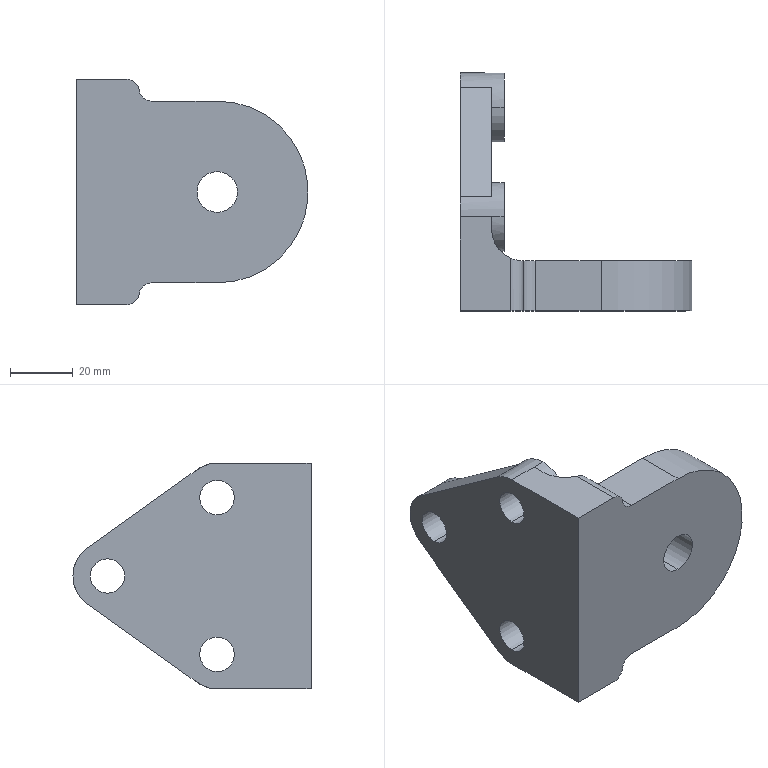Part | SolidWorks | features BaseBody 1 | 1 solid | 38 faces | box 74 x 76 x 72 mm | volume 94781 mm3 | cylinder 22 | plane 16 | commonest cylinder face diameters 11 x6 22 x6 8 x4 13 x2 36 x2 20 x1
STEP:
#1=CARTESIAN_POINT('',(45.,0.,42.5));
#2=VERTEX_POINT('',#1);
#3=CARTESIAN_POINT('',(45.,0.,29.5));
#4=VERTEX_POINT('',#3);
#5=CARTESIAN_POINT('',(45.,0.,36.));
#6=DIRECTION('',(0.,-1.,0.));
#7=DIRECTION('',(0.,0.,1.));
#8=AXIS2_PLACEMENT_3D('',#5,#6,#7);
#9=CIRCLE('',#8,6.5);
#10=EDGE_CURVE('',#2,#4,#9,.T.);
#11=ORIENTED_EDGE('',*,*,#10,.T.);
#12=CARTESIAN_POINT('',(45.,13.,29.5));
#13=VERTEX_POINT('',#12);
#14=CARTESIAN_POINT('',(45.,0.,29.5));
#15=DIRECTION('',(0.,1.,0.));
#16=VECTOR('',#15,1000.);
#17=LINE('',#14,#16);
#18=EDGE_CURVE('',#4,#13,#17,.T.);
#19=ORIENTED_EDGE('',*,*,#18,.T.);
#20=CARTESIAN_POINT('',(45.,13.,42.5));
#21=VERTEX_POINT('',#20);
#22=CARTESIAN_POINT('',(45.,13.,36.));
#23=DIRECTION('',(0.,-1.,0.));
#24=DIRECTION('',(0.,0.,1.));
#25=AXIS2_PLACEMENT_3D('',#22,#23,#24);
#26=CIRCLE('',#25,6.5);
#27=EDGE_CURVE('',#21,#13,#26,.T.);
#28=ORIENTED_EDGE('',*,*,#27,.F.);
#29=CARTESIAN_POINT('',(45.,0.,42.5));
#30=DIRECTION('',(0.,1.,0.));
#31=VECTOR('',#30,1000.);
#32=LINE('',#29,#31);
#33=EDGE_CURVE('',#2,#21,#32,.T.);
#34=ORIENTED_EDGE('',*,*,#33,.F.);
#35=EDGE_LOOP('',(#11,#19,#28,#34));
#36=FACE_OUTER_BOUND('',#35,.T.);
#37=CARTESIAN_POINT('',(45.,0.,36.));
#38=DIRECTION('',(0.,1.,0.));
#39=DIRECTION('',(0.,0.,1.));
#40=AXIS2_PLACEMENT_3D('',#37,#38,#39);
#41=CYLINDRICAL_SURFACE('',#40,6.5);
#42=ADVANCED_FACE('',(#36),#41,.F.);
#43=CARTESIAN_POINT('',(10.,30.,72.));
#44=VERTEX_POINT('',#43);
#45=CARTESIAN_POINT('',(0.,30.,72.));
#46=VERTEX_POINT('',#45);
#47=CARTESIAN_POINT('',(8.031,30.,72.));
#48=DIRECTION('',(-1.,0.,0.));
#49=VECTOR('',#48,1000.);
#50=LINE('',#47,#49);
#51=EDGE_CURVE('',#44,#46,#50,.T.);
#52=ORIENTED_EDGE('',*,*,#51,.F.);
#53=CARTESIAN_POINT('',(14.,30.,72.));
#54=VERTEX_POINT('',#53);
#55=CARTESIAN_POINT('',(0.,30.,72.));
#56=DIRECTION('',(1.,0.,0.));
#57=VECTOR('',#56,1000.);
#58=LINE('',#55,#57);
#59=EDGE_CURVE('',#44,#54,#58,.T.);
#60=ORIENTED_EDGE('',*,*,#59,.T.);
#61=CARTESIAN_POINT('',(14.,30.,50.));
#62=VERTEX_POINT('',#61);
#63=CARTESIAN_POINT('',(14.,30.,61.));
#64=DIRECTION('',(-1.,0.,0.));
#65=DIRECTION('',(0.,0.,-1.));
#66=AXIS2_PLACEMENT_3D('',#63,#64,#65);
#67=CIRCLE('',#66,11.);
#68=EDGE_CURVE('',#54,#62,#67,.T.);
#69=ORIENTED_EDGE('',*,*,#68,.T.);
#70=CARTESIAN_POINT('',(10.,30.,50.));
#71=VERTEX_POINT('',#70);
#72=CARTESIAN_POINT('',(0.,30.,50.));
#73=DIRECTION('',(1.,0.,0.));
#74=VECTOR('',#73,1000.);
#75=LINE('',#72,#74);
#76=EDGE_CURVE('',#71,#62,#75,.T.);
#77=ORIENTED_EDGE('',*,*,#76,.F.);
#78=CARTESIAN_POINT('',(10.,36.394,69.951));
#79=VERTEX_POINT('',#78);
#80=CARTESIAN_POINT('',(10.,30.,61.));
#81=DIRECTION('',(1.,0.,0.));
#82=DIRECTION('',(0.,0.,-1.));
#83=AXIS2_PLACEMENT_3D('',#80,#81,#82);
#84=CIRCLE('',#83,11.);
#85=EDGE_CURVE('',#71,#79,#84,.T.);
#86=ORIENTED_EDGE('',*,*,#85,.T.);
#87=CARTESIAN_POINT('',(0.,36.394,69.951));
#88=VERTEX_POINT('',#87);
#89=CARTESIAN_POINT('',(0.,36.394,69.951));
#90=DIRECTION('',(-1.,0.,0.));
#91=VECTOR('',#90,1000.);
#92=LINE('',#89,#91);
#93=EDGE_CURVE('',#79,#88,#92,.T.);
#94=ORIENTED_EDGE('',*,*,#93,.T.);
#95=CARTESIAN_POINT('',(0.,30.,61.));
#96=DIRECTION('',(1.,0.,0.));
#97=DIRECTION('',(0.,0.,-1.));
#98=AXIS2_PLACEMENT_3D('',#95,#96,#97);
#99=CIRCLE('',#98,11.);
#100=EDGE_CURVE('',#88,#46,#99,.T.);
#101=ORIENTED_EDGE('',*,*,#100,.T.);
#102=EDGE_LOOP('',(#52,#60,#69,#77,#86,#94,#101));
#103=FACE_OUTER_BOUND('',#102,.T.);
#104=CARTESIAN_POINT('',(0.,30.,61.));
#105=DIRECTION('',(1.,0.,0.));
#106=DIRECTION('',(0.,0.,-1.));
#107=AXIS2_PLACEMENT_3D('',#104,#105,#106);
#108=CYLINDRICAL_SURFACE('',#107,11.);
#109=ADVANCED_FACE('',(#103),#108,.T.);
#110=CARTESIAN_POINT('',(0.,65.,30.5));
#111=VERTEX_POINT('',#110);
#112=CARTESIAN_POINT('',(0.,65.,41.5));
#113=VERTEX_POINT('',#112);
#114=CARTESIAN_POINT('',(0.,65.,36.));
#115=DIRECTION('',(-1.,0.,0.));
#116=DIRECTION('',(0.,0.,-1.));
#117=AXIS2_PLACEMENT_3D('',#114,#115,#116);
#118=CIRCLE('',#117,5.5);
#119=EDGE_CURVE('',#111,#113,#118,.T.);
#120=ORIENTED_EDGE('',*,*,#119,.T.);
#121=CARTESIAN_POINT('',(14.,65.,41.5));
#122=VERTEX_POINT('',#121);
#123=CARTESIAN_POINT('',(0.,65.,41.5));
#124=DIRECTION('',(1.,0.,0.));
#125=VECTOR('',#124,1000.);
#126=LINE('',#123,#125);
#127=EDGE_CURVE('',#113,#122,#126,.T.);
#128=ORIENTED_EDGE('',*,*,#127,.T.);
#129=CARTESIAN_POINT('',(14.,65.,30.5));
#130=VERTEX_POINT('',#129);
#131=CARTESIAN_POINT('',(14.,65.,36.));
#132=DIRECTION('',(-1.,0.,0.));
#133=DIRECTION('',(0.,0.,-1.));
#134=AXIS2_PLACEMENT_3D('',#131,#132,#133);
#135=CIRCLE('',#134,5.5);
#136=EDGE_CURVE('',#130,#122,#135,.T.);
#137=ORIENTED_EDGE('',*,*,#136,.F.);
#138=CARTESIAN_POINT('',(0.,65.,30.5));
#139=DIRECTION('',(1.,0.,0.));
#140=VECTOR('',#139,1000.);
#141=LINE('',#138,#140);
#142=EDGE_CURVE('',#111,#130,#141,.T.);
#143=ORIENTED_EDGE('',*,*,#142,.F.);
#144=EDGE_LOOP('',(#120,#128,#137,#143));
#145=FACE_OUTER_BOUND('',#144,.T.);
#146=CARTESIAN_POINT('',(0.,65.,36.));
#147=DIRECTION('',(1.,0.,0.));
#148=DIRECTION('',(0.,0.,-1.));
#149=AXIS2_PLACEMENT_3D('',#146,#147,#148);
#150=CYLINDRICAL_SURFACE('',#149,5.5);
#151=ADVANCED_FACE('',(#145),#150,.F.);
#152=CARTESIAN_POINT('',(0.,30.,55.5));
#153=VERTEX_POINT('',#152);
#154=CARTESIAN_POINT('',(0.,30.,66.5));
#155=VERTEX_POINT('',#154);
#156=CARTESIAN_POINT('',(0.,30.,61.));
#157=DIRECTION('',(-1.,0.,0.));
#158=DIRECTION('',(0.,0.,-1.));
#159=AXIS2_PLACEMENT_3D('',#156,#157,#158);
#160=CIRCLE('',#159,5.5);
#161=EDGE_CURVE('',#153,#155,#160,.T.);
#162=ORIENTED_EDGE('',*,*,#161,.T.);
#163=CARTESIAN_POINT('',(14.,30.,66.5));
#164=VERTEX_POINT('',#163);
#165=CARTESIAN_POINT('',(0.,30.,66.5));
#166=DIRECTION('',(1.,0.,0.));
#167=VECTOR('',#166,1000.);
#168=LINE('',#165,#167);
#169=EDGE_CURVE('',#155,#164,#168,.T.);
#170=ORIENTED_EDGE('',*,*,#169,.T.);
#171=CARTESIAN_POINT('',(14.,30.,55.5));
#172=VERTEX_POINT('',#171);
#173=CARTESIAN_POINT('',(14.,30.,61.));
#174=DIRECTION('',(-1.,0.,0.));
#175=DIRECTION('',(0.,0.,-1.));
#176=AXIS2_PLACEMENT_3D('',#173,#174,#175);
#177=CIRCLE('',#176,5.5);
#178=EDGE_CURVE('',#172,#164,#177,.T.);
#179=ORIENTED_EDGE('',*,*,#178,.F.);
#180=CARTESIAN_POINT('',(0.,30.,55.5));
#181=DIRECTION('',(1.,0.,0.));
#182=VECTOR('',#181,1000.);
#183=LINE('',#180,#182);
#184=EDGE_CURVE('',#153,#172,#183,.T.);
#185=ORIENTED_EDGE('',*,*,#184,.F.);
#186=EDGE_LOOP('',(#162,#170,#179,#185));
#187=FACE_OUTER_BOUND('',#186,.T.);
#188=CARTESIAN_POINT('',(0.,30.,61.));
#189=DIRECTION('',(1.,0.,0.));
#190=DIRECTION('',(0.,0.,-1.));
#191=AXIS2_PLACEMENT_3D('',#188,#189,#190);
#192=CYLINDRICAL_SURFACE('',#191,5.5);
#193=ADVANCED_FACE('',(#187),#192,.F.);
#194=CARTESIAN_POINT('',(0.,30.,5.5));
#195=VERTEX_POINT('',#194);
#196=CARTESIAN_POINT('',(0.,30.,16.5));
#197=VERTEX_POINT('',#196);
#198=CARTESIAN_POINT('',(0.,30.,11.));
#199=DIRECTION('',(-1.,0.,0.));
#200=DIRECTION('',(0.,0.,-1.));
#201=AXIS2_PLACEMENT_3D('',#198,#199,#200);
#202=CIRCLE('',#201,5.5);
#203=EDGE_CURVE('',#195,#197,#202,.T.);
#204=ORIENTED_EDGE('',*,*,#203,.T.);
#205=CARTESIAN_POINT('',(14.,30.,16.5));
#206=VERTEX_POINT('',#205);
#207=CARTESIAN_POINT('',(0.,30.,16.5));
#208=DIRECTION('',(1.,0.,0.));
#209=VECTOR('',#208,1000.);
#210=LINE('',#207,#209);
#211=EDGE_CURVE('',#197,#206,#210,.T.);
#212=ORIENTED_EDGE('',*,*,#211,.T.);
#213=CARTESIAN_POINT('',(14.,30.,5.5));
#214=VERTEX_POINT('',#213);
#215=CARTESIAN_POINT('',(14.,30.,11.));
#216=DIRECTION('',(-1.,0.,0.));
#217=DIRECTION('',(0.,0.,-1.));
#218=AXIS2_PLACEMENT_3D('',#215,#216,#217);
#219=CIRCLE('',#218,5.5);
#220=EDGE_CURVE('',#214,#206,#219,.T.);
#221=ORIENTED_EDGE('',*,*,#220,.F.);
#222=CARTESIAN_POINT('',(0.,30.,5.5));
#223=DIRECTION('',(1.,0.,0.));
#224=VECTOR('',#223,1000.);
#225=LINE('',#222,#224);
#226=EDGE_CURVE('',#195,#214,#225,.T.);
#227=ORIENTED_EDGE('',*,*,#226,.F.);
#228=EDGE_LOOP('',(#204,#212,#221,#227));
#229=FACE_OUTER_BOUND('',#228,.T.);
#230=CARTESIAN_POINT('',(0.,30.,11.));
#231=DIRECTION('',(1.,0.,0.));
#232=DIRECTION('',(0.,0.,-1.));
#233=AXIS2_PLACEMENT_3D('',#230,#231,#232);
#234=CYLINDRICAL_SURFACE('',#233,5.5);
#235=ADVANCED_FACE('',(#229),#234,.F.);
#236=CARTESIAN_POINT('',(10.,36.394,2.049));
#237=VERTEX_POINT('',#236);
#238=CARTESIAN_POINT('',(10.,30.,22.));
#239=VERTEX_POINT('',#238);
#240=CARTESIAN_POINT('',(10.,30.,11.));
#241=DIRECTION('',(1.,0.,0.));
#242=DIRECTION('',(0.,0.,-1.));
#243=AXIS2_PLACEMENT_3D('',#240,#241,#242);
#244=CIRCLE('',#243,11.);
#245=EDGE_CURVE('',#237,#239,#244,.T.);
#246=ORIENTED_EDGE('',*,*,#245,.T.);
#247=CARTESIAN_POINT('',(14.,30.,22.));
#248=VERTEX_POINT('',#247);
#249=CARTESIAN_POINT('',(0.,30.,22.));
#250=DIRECTION('',(1.,0.,0.));
#251=VECTOR('',#250,1000.);
#252=LINE('',#249,#251);
#253=EDGE_CURVE('',#239,#248,#252,.T.);
#254=ORIENTED_EDGE('',*,*,#253,.T.);
#255=CARTESIAN_POINT('',(14.,30.,0.));
#256=VERTEX_POINT('',#255);
#257=CARTESIAN_POINT('',(14.,30.,11.));
#258=DIRECTION('',(-1.,0.,0.));
#259=DIRECTION('',(0.,0.,-1.));
#260=AXIS2_PLACEMENT_3D('',#257,#258,#259);
#261=CIRCLE('',#260,11.);
#262=EDGE_CURVE('',#248,#256,#261,.T.);
#263=ORIENTED_EDGE('',*,*,#262,.T.);
#264=CARTESIAN_POINT('',(10.,30.,0.));
#265=VERTEX_POINT('',#264);
#266=CARTESIAN_POINT('',(0.,30.,0.));
#267=DIRECTION('',(1.,0.,0.));
#268=VECTOR('',#267,1000.);
#269=LINE('',#266,#268);
#270=EDGE_CURVE('',#265,#256,#269,.T.);
#271=ORIENTED_EDGE('',*,*,#270,.F.);
#272=CARTESIAN_POINT('',(0.,30.,0.));
#273=VERTEX_POINT('',#272);
#274=CARTESIAN_POINT('',(8.031,30.,0.));
#275=DIRECTION('',(-1.,0.,0.));
#276=VECTOR('',#275,1000.);
#277=LINE('',#274,#276);
#278=EDGE_CURVE('',#265,#273,#277,.T.);
#279=ORIENTED_EDGE('',*,*,#278,.T.);
#280=CARTESIAN_POINT('',(0.,36.394,2.049));
#281=VERTEX_POINT('',#280);
#282=CARTESIAN_POINT('',(0.,30.,11.));
#283=DIRECTION('',(1.,0.,0.));
#284=DIRECTION('',(0.,0.,-1.));
#285=AXIS2_PLACEMENT_3D('',#282,#283,#284);
#286=CIRCLE('',#285,11.);
#287=EDGE_CURVE('',#273,#281,#286,.T.);
#288=ORIENTED_EDGE('',*,*,#287,.T.);
#289=CARTESIAN_POINT('',(0.,36.394,2.049));
#290=DIRECTION('',(1.,0.,0.));
#291=VECTOR('',#290,1000.);
#292=LINE('',#289,#291);
#293=EDGE_CURVE('',#281,#237,#292,.T.);
#294=ORIENTED_EDGE('',*,*,#293,.T.);
#295=EDGE_LOOP('',(#246,#254,#263,#271,#279,#288,#294));
#296=FACE_OUTER_BOUND('',#295,.T.);
#297=CARTESIAN_POINT('',(0.,30.,11.));
#298=DIRECTION('',(1.,0.,0.));
#299=DIRECTION('',(0.,0.,-1.));
#300=AXIS2_PLACEMENT_3D('',#297,#298,#299);
#301=CYLINDRICAL_SURFACE('',#300,11.);
#302=ADVANCED_FACE('',(#296),#301,.T.);
#303=CARTESIAN_POINT('',(10.,71.394,44.951));
#304=VERTEX_POINT('',#303);
#305=CARTESIAN_POINT('',(10.,65.,47.));
#306=VERTEX_POINT('',#305);
#307=CARTESIAN_POINT('',(10.,65.,36.));
#308=DIRECTION('',(1.,0.,0.));
#309=DIRECTION('',(0.,0.,-1.));
#310=AXIS2_PLACEMENT_3D('',#307,#308,#309);
#311=CIRCLE('',#310,11.);
#312=EDGE_CURVE('',#304,#306,#311,.T.);
#313=ORIENTED_EDGE('',*,*,#312,.T.);
#314=CARTESIAN_POINT('',(14.,65.,47.));
#315=VERTEX_POINT('',#314);
#316=CARTESIAN_POINT('',(0.,65.,47.));
#317=DIRECTION('',(1.,0.,0.));
#318=VECTOR('',#317,1000.);
#319=LINE('',#316,#318);
#320=EDGE_CURVE('',#306,#315,#319,.T.);
#321=ORIENTED_EDGE('',*,*,#320,.T.);
#322=CARTESIAN_POINT('',(14.,65.,25.));
#323=VERTEX_POINT('',#322);
#324=CARTESIAN_POINT('',(14.,65.,36.));
#325=DIRECTION('',(-1.,0.,0.));
#326=DIRECTION('',(0.,0.,-1.));
#327=AXIS2_PLACEMENT_3D('',#324,#325,#326);
#328=CIRCLE('',#327,11.);
#329=EDGE_CURVE('',#315,#323,#328,.T.);
#330=ORIENTED_EDGE('',*,*,#329,.T.);
#331=CARTESIAN_POINT('',(10.,65.,25.));
#332=VERTEX_POINT('',#331);
#333=CARTESIAN_POINT('',(0.,65.,25.));
#334=DIRECTION('',(1.,0.,0.));
#335=VECTOR('',#334,1000.);
#336=LINE('',#333,#335);
#337=EDGE_CURVE('',#332,#323,#336,.T.);
#338=ORIENTED_EDGE('',*,*,#337,.F.);
#339=CARTESIAN_POINT('',(10.,71.394,27.049));
#340=VERTEX_POINT('',#339);
#341=CARTESIAN_POINT('',(10.,65.,36.));
#342=DIRECTION('',(1.,0.,0.));
#343=DIRECTION('',(0.,0.,-1.));
#344=AXIS2_PLACEMENT_3D('',#341,#342,#343);
#345=CIRCLE('',#344,11.);
#346=EDGE_CURVE('',#332,#340,#345,.T.);
#347=ORIENTED_EDGE('',*,*,#346,.T.);
#348=CARTESIAN_POINT('',(0.,71.394,27.049));
#349=VERTEX_POINT('',#348);
#350=CARTESIAN_POINT('',(0.,71.394,27.049));
#351=DIRECTION('',(-1.,0.,0.));
#352=VECTOR('',#351,1000.);
#353=LINE('',#350,#352);
#354=EDGE_CURVE('',#340,#349,#353,.T.);
#355=ORIENTED_EDGE('',*,*,#354,.T.);
#356=CARTESIAN_POINT('',(0.,71.394,44.951));
#357=VERTEX_POINT('',#356);
#358=CARTESIAN_POINT('',(0.,65.,36.));
#359=DIRECTION('',(1.,0.,0.));
#360=DIRECTION('',(0.,0.,-1.));
#361=AXIS2_PLACEMENT_3D('',#358,#359,#360);
#362=CIRCLE('',#361,11.);
#363=EDGE_CURVE('',#349,#357,#362,.T.);
#364=ORIENTED_EDGE('',*,*,#363,.T.);
#365=CARTESIAN_POINT('',(5.,71.394,44.951));
#366=DIRECTION('',(-1.,0.,0.));
#367=VECTOR('',#366,1000.);
#368=LINE('',#365,#367);
#369=EDGE_CURVE('',#304,#357,#368,.T.);
#370=ORIENTED_EDGE('',*,*,#369,.F.);
#371=EDGE_LOOP('',(#313,#321,#330,#338,#347,#355,#364,#370));
#372=FACE_OUTER_BOUND('',#371,.T.);
#373=CARTESIAN_POINT('',(0.,65.,36.));
#374=DIRECTION('',(1.,0.,0.));
#375=DIRECTION('',(0.,0.,-1.));
#376=AXIS2_PLACEMENT_3D('',#373,#374,#375);
#377=CYLINDRICAL_SURFACE('',#376,11.);
#378=ADVANCED_FACE('',(#372),#377,.T.);
#379=CARTESIAN_POINT('',(45.,13.,18.));
#380=VERTEX_POINT('',#379);
#381=CARTESIAN_POINT('',(45.,13.,54.));
#382=VERTEX_POINT('',#381);
#383=CARTESIAN_POINT('',(45.,13.,36.));
#384=DIRECTION('',(0.,1.,0.));
#385=DIRECTION('',(0.,0.,1.));
#386=AXIS2_PLACEMENT_3D('',#383,#384,#385);
#387=CIRCLE('',#386,18.);
#388=EDGE_CURVE('',#380,#382,#387,.T.);
#389=ORIENTED_EDGE('',*,*,#388,.F.);
#390=CARTESIAN_POINT('',(45.,16.,18.));
#391=VERTEX_POINT('',#390);
#392=CARTESIAN_POINT('',(45.,13.,18.));
#393=DIRECTION('',(0.,1.,0.));
#394=VECTOR('',#393,1000.);
#395=LINE('',#392,#394);
#396=EDGE_CURVE('',#380,#391,#395,.T.);
#397=ORIENTED_EDGE('',*,*,#396,.T.);
#398=CARTESIAN_POINT('',(45.,16.,54.));
#399=VERTEX_POINT('',#398);
#400=CARTESIAN_POINT('',(45.,16.,36.));
#401=DIRECTION('',(0.,-1.,0.));
#402=DIRECTION('',(0.,0.,1.));
#403=AXIS2_PLACEMENT_3D('',#400,#401,#402);
#404=CIRCLE('',#403,18.);
#405=EDGE_CURVE('',#399,#391,#404,.T.);
#406=ORIENTED_EDGE('',*,*,#405,.F.);
#407=CARTESIAN_POINT('',(45.,13.,54.));
#408=DIRECTION('',(0.,1.,0.));
#409=VECTOR('',#408,1000.);
#410=LINE('',#407,#409);
#411=EDGE_CURVE('',#382,#399,#410,.T.);
#412=ORIENTED_EDGE('',*,*,#411,.F.);
#413=EDGE_LOOP('',(#389,#397,#406,#412));
#414=FACE_OUTER_BOUND('',#413,.T.);
#415=CARTESIAN_POINT('',(45.,13.,36.));
#416=DIRECTION('',(0.,1.,0.));
#417=DIRECTION('',(0.,0.,1.));
#418=AXIS2_PLACEMENT_3D('',#415,#416,#417);
#419=CYLINDRICAL_SURFACE('',#418,18.);
#420=ADVANCED_FACE('',(#414),#419,.F.);
#421=ORIENTED_EDGE('',*,*,#10,.F.);
#422=CARTESIAN_POINT('',(45.,0.,36.));
#423=DIRECTION('',(0.,-1.,0.));
#424=DIRECTION('',(0.,0.,1.));
#425=AXIS2_PLACEMENT_3D('',#422,#423,#424);
#426=CIRCLE('',#425,6.5);
#427=EDGE_CURVE('',#4,#2,#426,.T.);
#428=ORIENTED_EDGE('',*,*,#427,.F.);
#429=EDGE_LOOP('',(#421,#428));
#430=FACE_BOUND('',#429,.T.);
#431=CARTESIAN_POINT('',(16.063,0.,72.));
#432=VERTEX_POINT('',#431);
#433=CARTESIAN_POINT('',(20.031,0.,68.5));
#434=VERTEX_POINT('',#433);
#435=CARTESIAN_POINT('',(16.063,0.,68.));
#436=DIRECTION('',(0.,1.,0.));
#437=DIRECTION('',(0.,0.,-1.));
#438=AXIS2_PLACEMENT_3D('',#435,#436,#437);
#439=CIRCLE('',#438,4.);
#440=EDGE_CURVE('',#432,#434,#439,.T.);
#441=ORIENTED_EDGE('',*,*,#440,.F.);
#442=CARTESIAN_POINT('',(0.,0.,72.));
#443=VERTEX_POINT('',#442);
#444=CARTESIAN_POINT('',(37.012,0.,72.));
#445=DIRECTION('',(1.,0.,0.));
#446=VECTOR('',#445,1000.);
#447=LINE('',#444,#446);
#448=EDGE_CURVE('',#443,#432,#447,.T.);
#449=ORIENTED_EDGE('',*,*,#448,.F.);
#450=CARTESIAN_POINT('',(0.,0.,0.));
#451=VERTEX_POINT('',#450);
#452=CARTESIAN_POINT('',(0.,0.,36.));
#453=DIRECTION('',(0.,0.,1.));
#454=VECTOR('',#453,1000.);
#455=LINE('',#452,#454);
#456=EDGE_CURVE('',#451,#443,#455,.T.);
#457=ORIENTED_EDGE('',*,*,#456,.F.);
#458=CARTESIAN_POINT('',(16.063,0.,0.));
#459=VERTEX_POINT('',#458);
#460=CARTESIAN_POINT('',(37.012,0.,0.));
#461=DIRECTION('',(-1.,0.,0.));
#462=VECTOR('',#461,1000.);
#463=LINE('',#460,#462);
#464=EDGE_CURVE('',#459,#451,#463,.T.);
#465=ORIENTED_EDGE('',*,*,#464,.F.);
#466=CARTESIAN_POINT('',(20.031,0.,3.5));
#467=VERTEX_POINT('',#466);
#468=CARTESIAN_POINT('',(16.063,0.,4.));
#469=DIRECTION('',(0.,1.,0.));
#470=DIRECTION('',(0.,0.,1.));
#471=AXIS2_PLACEMENT_3D('',#468,#469,#470);
#472=CIRCLE('',#471,4.);
#473=EDGE_CURVE('',#467,#459,#472,.T.);
#474=ORIENTED_EDGE('',*,*,#473,.F.);
#475=CARTESIAN_POINT('',(24.,0.,7.));
#476=VERTEX_POINT('',#475);
#477=CARTESIAN_POINT('',(24.,0.,3.));
#478=DIRECTION('',(0.,-1.,0.));
#479=DIRECTION('',(0.,0.,1.));
#480=AXIS2_PLACEMENT_3D('',#477,#478,#479);
#481=CIRCLE('',#480,4.);
#482=EDGE_CURVE('',#476,#467,#481,.T.);
#483=ORIENTED_EDGE('',*,*,#482,.F.);
#484=CARTESIAN_POINT('',(45.,0.,7.));
#485=VERTEX_POINT('',#484);
#486=CARTESIAN_POINT('',(37.012,0.,7.));
#487=DIRECTION('',(-1.,0.,0.));
#488=VECTOR('',#487,1000.);
#489=LINE('',#486,#488);
#490=EDGE_CURVE('',#485,#476,#489,.T.);
#491=ORIENTED_EDGE('',*,*,#490,.F.);
#492=CARTESIAN_POINT('',(45.,0.,65.));
#493=VERTEX_POINT('',#492);
#494=CARTESIAN_POINT('',(45.,0.,36.));
#495=DIRECTION('',(0.,1.,0.));
#496=DIRECTION('',(0.,0.,1.));
#497=AXIS2_PLACEMENT_3D('',#494,#495,#496);
#498=CIRCLE('',#497,29.);
#499=EDGE_CURVE('',#493,#485,#498,.T.);
#500=ORIENTED_EDGE('',*,*,#499,.F.);
#501=CARTESIAN_POINT('',(24.,0.,65.));
#502=VERTEX_POINT('',#501);
#503=CARTESIAN_POINT('',(37.012,0.,65.));
#504=DIRECTION('',(1.,0.,0.));
#505=VECTOR('',#504,1000.);
#506=LINE('',#503,#505);
#507=EDGE_CURVE('',#502,#493,#506,.T.);
#508=ORIENTED_EDGE('',*,*,#507,.F.);
#509=CARTESIAN_POINT('',(24.,0.,69.));
#510=DIRECTION('',(0.,-1.,0.));
#511=DIRECTION('',(0.,0.,-1.));
#512=AXIS2_PLACEMENT_3D('',#509,#510,#511);
#513=CIRCLE('',#512,4.);
#514=EDGE_CURVE('',#434,#502,#513,.T.);
#515=ORIENTED_EDGE('',*,*,#514,.F.);
#516=EDGE_LOOP('',(#441,#449,#457,#465,#474,#483,#491,#500,#508,#515));
#517=FACE_OUTER_BOUND('',#516,.T.);
#518=CARTESIAN_POINT('',(37.012,0.,36.));
#519=DIRECTION('',(0.,1.,0.));
#520=DIRECTION('',(0.,0.,1.));
#521=AXIS2_PLACEMENT_3D('',#518,#519,#520);
#522=PLANE('',#521);
#523=ADVANCED_FACE('',(#430,#517),#522,.F.);
#524=ORIENTED_EDGE('',*,*,#18,.F.);
#525=ORIENTED_EDGE('',*,*,#427,.T.);
#526=ORIENTED_EDGE('',*,*,#33,.T.);
#527=CARTESIAN_POINT('',(45.,13.,36.));
#528=DIRECTION('',(0.,-1.,0.));
#529=DIRECTION('',(0.,0.,1.));
#530=AXIS2_PLACEMENT_3D('',#527,#528,#529);
#531=CIRCLE('',#530,6.5);
#532=EDGE_CURVE('',#13,#21,#531,.T.);
#533=ORIENTED_EDGE('',*,*,#532,.F.);
#534=EDGE_LOOP('',(#524,#525,#526,#533));
#535=FACE_OUTER_BOUND('',#534,.T.);
#536=CARTESIAN_POINT('',(45.,0.,36.));
#537=DIRECTION('',(0.,1.,0.));
#538=DIRECTION('',(0.,0.,1.));
#539=AXIS2_PLACEMENT_3D('',#536,#537,#538);
#540=CYLINDRICAL_SURFACE('',#539,6.5);
#541=ADVANCED_FACE('',(#535),#540,.F.);
#542=CARTESIAN_POINT('',(20.031,16.,68.5));
#543=VERTEX_POINT('',#542);
#544=CARTESIAN_POINT('',(20.031,16.,68.5));
#545=DIRECTION('',(0.,1.,0.));
#546=VECTOR('',#545,1000.);
#547=LINE('',#544,#546);
#548=EDGE_CURVE('',#434,#543,#547,.T.);
#549=ORIENTED_EDGE('',*,*,#548,.F.);
#550=ORIENTED_EDGE('',*,*,#514,.T.);
#551=CARTESIAN_POINT('',(24.,16.,65.));
#552=VERTEX_POINT('',#551);
#553=CARTESIAN_POINT('',(24.,8.,65.));
#554=DIRECTION('',(0.,-1.,0.));
#555=VECTOR('',#554,1000.);
#556=LINE('',#553,#555);
#557=EDGE_CURVE('',#552,#502,#556,.T.);
#558=ORIENTED_EDGE('',*,*,#557,.F.);
#559=CARTESIAN_POINT('',(24.,16.,69.));
#560=DIRECTION('',(0.,-1.,0.));
#561=DIRECTION('',(0.,0.,-1.));
#562=AXIS2_PLACEMENT_3D('',#559,#560,#561);
#563=CIRCLE('',#562,4.);
#564=EDGE_CURVE('',#543,#552,#563,.T.);
#565=ORIENTED_EDGE('',*,*,#564,.F.);
#566=EDGE_LOOP('',(#549,#550,#558,#565));
#567=FACE_OUTER_BOUND('',#566,.T.);
#568=CARTESIAN_POINT('',(24.,16.,69.));
#569=DIRECTION('',(0.,-1.,0.));
#570=DIRECTION('',(0.,0.,-1.));
#571=AXIS2_PLACEMENT_3D('',#568,#569,#570);
#572=CYLINDRICAL_SURFACE('',#571,4.);
#573=ADVANCED_FACE('',(#567),#572,.F.);
#574=CARTESIAN_POINT('',(16.063,16.808,72.));
#575=VERTEX_POINT('',#574);
#576=CARTESIAN_POINT('',(16.063,16.909,72.));
#577=DIRECTION('',(0.,-1.,0.));
#578=VECTOR('',#577,1000.);
#579=LINE('',#576,#578);
#580=EDGE_CURVE('',#575,#432,#579,.T.);
#581=ORIENTED_EDGE('',*,*,#580,.T.);
#582=ORIENTED_EDGE('',*,*,#440,.T.);
#583=ORIENTED_EDGE('',*,*,#548,.T.);
#584=CARTESIAN_POINT('',(20.,16.,68.706));
#585=VERTEX_POINT('',#584);
#586=CARTESIAN_POINT('',(16.063,16.,68.));
#587=DIRECTION('',(0.,-1.,0.));
#588=DIRECTION('',(0.,0.,-1.));
#589=AXIS2_PLACEMENT_3D('',#586,#587,#588);
#590=CIRCLE('',#589,4.);
#591=EDGE_CURVE('',#543,#585,#590,.T.);
#592=ORIENTED_EDGE('',*,*,#591,.T.);
#593=CARTESIAN_POINT('',(20.,16.,68.706));
#594=CARTESIAN_POINT('',(19.958,16.,68.941));
#595=CARTESIAN_POINT('',(19.896,16.,69.168));
#596=CARTESIAN_POINT('',(19.732,16.003,69.61));
#597=CARTESIAN_POINT('',(19.63,16.006,69.825));
#598=CARTESIAN_POINT('',(19.389,16.018,70.234));
#599=CARTESIAN_POINT('',(19.252,16.027,70.426));
#600=CARTESIAN_POINT('',(18.946,16.055,70.783));
#601=CARTESIAN_POINT('',(18.775,16.074,70.949));
#602=CARTESIAN_POINT('',(18.41,16.125,71.247));
#603=CARTESIAN_POINT('',(18.217,16.158,71.378));
#604=CARTESIAN_POINT('',(17.812,16.24,71.605));
#605=CARTESIAN_POINT('',(17.598,16.29,71.701));
#606=CARTESIAN_POINT('',(17.165,16.408,71.852));
#607=CARTESIAN_POINT('',(16.946,16.475,71.908));
#608=CARTESIAN_POINT('',(16.505,16.628,71.982));
#609=CARTESIAN_POINT('',(16.282,16.714,72.));
#610=CARTESIAN_POINT('',(16.063,16.808,72.));
#611=B_SPLINE_CURVE_WITH_KNOTS('',3,(#593,#594,#595,#596,#597,#598,#599,#600,#601,#602,#603,#604,#605,#606,#607,#608,#609,#610),.UNSPECIFIED.,.F.,.F.,(4,2,2,2,2,2,2,2,4),(0.,0.000706,0.001412,0.002118,0.002824,0.00353,0.004236,0.004942,0.005648),.UNSPECIFIED.);
#612=EDGE_CURVE('',#585,#575,#611,.T.);
#613=ORIENTED_EDGE('',*,*,#612,.T.);
#614=EDGE_LOOP('',(#581,#582,#583,#592,#613));
#615=FACE_OUTER_BOUND('',#614,.T.);
#616=CARTESIAN_POINT('',(16.063,16.909,68.));
#617=DIRECTION('',(0.,-1.,0.));
#618=DIRECTION('',(0.,0.,-1.));
#619=AXIS2_PLACEMENT_3D('',#616,#617,#618);
#620=CYLINDRICAL_SURFACE('',#619,4.);
#621=ADVANCED_FACE('',(#615),#620,.T.);
#622=ORIENTED_EDGE('',*,*,#51,.T.);
#623=CARTESIAN_POINT('',(0.,15.,72.));
#624=DIRECTION('',(0.,-1.,0.));
#625=VECTOR('',#624,1000.);
#626=LINE('',#623,#625);
#627=EDGE_CURVE('',#46,#443,#626,.T.);
#628=ORIENTED_EDGE('',*,*,#627,.T.);
#629=ORIENTED_EDGE('',*,*,#448,.T.);
#630=ORIENTED_EDGE('',*,*,#580,.F.);
#631=CARTESIAN_POINT('',(10.,26.,72.));
#632=VERTEX_POINT('',#631);
#633=CARTESIAN_POINT('',(20.,26.,72.));
#634=DIRECTION('',(0.,0.,-1.));
#635=DIRECTION('',(-1.,0.,0.));
#636=AXIS2_PLACEMENT_3D('',#633,#634,#635);
#637=CIRCLE('',#636,10.);
#638=EDGE_CURVE('',#575,#632,#637,.T.);
#639=ORIENTED_EDGE('',*,*,#638,.T.);
#640=CARTESIAN_POINT('',(10.,15.,72.));
#641=DIRECTION('',(0.,1.,0.));
#642=VECTOR('',#641,1000.);
#643=LINE('',#640,#642);
#644=EDGE_CURVE('',#632,#44,#643,.T.);
#645=ORIENTED_EDGE('',*,*,#644,.T.);
#646=EDGE_LOOP('',(#622,#628,#629,#630,#639,#645));
#647=FACE_OUTER_BOUND('',#646,.T.);
#648=CARTESIAN_POINT('',(8.031,15.,72.));
#649=DIRECTION('',(0.,0.,1.));
#650=DIRECTION('',(1.,0.,0.));
#651=AXIS2_PLACEMENT_3D('',#648,#649,#650);
#652=PLANE('',#651);
#653=ADVANCED_FACE('',(#647),#652,.T.);
#654=ORIENTED_EDGE('',*,*,#119,.F.);
#655=CARTESIAN_POINT('',(0.,65.,36.));
#656=DIRECTION('',(-1.,0.,0.));
#657=DIRECTION('',(0.,0.,-1.));
#658=AXIS2_PLACEMENT_3D('',#655,#656,#657);
#659=CIRCLE('',#658,5.5);
#660=EDGE_CURVE('',#113,#111,#659,.T.);
#661=ORIENTED_EDGE('',*,*,#660,.F.);
#662=EDGE_LOOP('',(#654,#661));
#663=FACE_BOUND('',#662,.T.);
#664=ORIENTED_EDGE('',*,*,#161,.F.);
#665=CARTESIAN_POINT('',(0.,30.,61.));
#666=DIRECTION('',(-1.,0.,0.));
#667=DIRECTION('',(0.,0.,-1.));
#668=AXIS2_PLACEMENT_3D('',#665,#666,#667);
#669=CIRCLE('',#668,5.5);
#670=EDGE_CURVE('',#155,#153,#669,.T.);
#671=ORIENTED_EDGE('',*,*,#670,.F.);
#672=EDGE_LOOP('',(#664,#671));
#673=FACE_BOUND('',#672,.T.);
#674=ORIENTED_EDGE('',*,*,#203,.F.);
#675=CARTESIAN_POINT('',(0.,30.,11.));
#676=DIRECTION('',(-1.,0.,0.));
#677=DIRECTION('',(0.,0.,-1.));
#678=AXIS2_PLACEMENT_3D('',#675,#676,#677);
#679=CIRCLE('',#678,5.5);
#680=EDGE_CURVE('',#197,#195,#679,.T.);
#681=ORIENTED_EDGE('',*,*,#680,.F.);
#682=EDGE_LOOP('',(#674,#681));
#683=FACE_BOUND('',#682,.T.);
#684=CARTESIAN_POINT('',(0.,38.,0.));
#685=DIRECTION('',(0.,1.,0.));
#686=VECTOR('',#685,1000.);
#687=LINE('',#684,#686);
#688=EDGE_CURVE('',#451,#273,#687,.T.);
#689=ORIENTED_EDGE('',*,*,#688,.F.);
#690=ORIENTED_EDGE('',*,*,#456,.T.);
#691=ORIENTED_EDGE('',*,*,#627,.F.);
#692=ORIENTED_EDGE('',*,*,#100,.F.);
#693=CARTESIAN_POINT('',(0.,71.394,44.951));
#694=DIRECTION('',(0.,-0.8137,0.5812));
#695=VECTOR('',#694,1000.);
#696=LINE('',#693,#695);
#697=EDGE_CURVE('',#357,#88,#696,.T.);
#698=ORIENTED_EDGE('',*,*,#697,.F.);
#699=ORIENTED_EDGE('',*,*,#363,.F.);
#700=CARTESIAN_POINT('',(0.,36.394,2.049));
#701=DIRECTION('',(0.,0.8137,0.5812));
#702=VECTOR('',#701,1000.);
#703=LINE('',#700,#702);
#704=EDGE_CURVE('',#281,#349,#703,.T.);
#705=ORIENTED_EDGE('',*,*,#704,.F.);
#706=ORIENTED_EDGE('',*,*,#287,.F.);
#707=EDGE_LOOP('',(#689,#690,#691,#692,#698,#699,#705,#706));
#708=FACE_OUTER_BOUND('',#707,.T.);
#709=CARTESIAN_POINT('',(0.,38.,36.));
#710=DIRECTION('',(1.,0.,0.));
#711=DIRECTION('',(0.,0.,-1.));
#712=AXIS2_PLACEMENT_3D('',#709,#710,#711);
#713=PLANE('',#712);
#714=ADVANCED_FACE('',(#663,#673,#683,#708),#713,.F.);
#715=ORIENTED_EDGE('',*,*,#464,.T.);
#716=ORIENTED_EDGE('',*,*,#688,.T.);
#717=ORIENTED_EDGE('',*,*,#278,.F.);
#718=CARTESIAN_POINT('',(10.,26.,0.));
#719=VERTEX_POINT('',#718);
#720=CARTESIAN_POINT('',(10.,15.,0.));
#721=DIRECTION('',(0.,1.,0.));
#722=VECTOR('',#721,1000.);
#723=LINE('',#720,#722);
#724=EDGE_CURVE('',#719,#265,#723,.T.);
#725=ORIENTED_EDGE('',*,*,#724,.F.);
#726=CARTESIAN_POINT('',(16.063,16.808,0.));
#727=VERTEX_POINT('',#726);
#728=CARTESIAN_POINT('',(20.,26.,0.));
#729=DIRECTION('',(0.,0.,-1.));
#730=DIRECTION('',(-1.,0.,0.));
#731=AXIS2_PLACEMENT_3D('',#728,#729,#730);
#732=CIRCLE('',#731,10.);
#733=EDGE_CURVE('',#727,#719,#732,.T.);
#734=ORIENTED_EDGE('',*,*,#733,.F.);
#735=CARTESIAN_POINT('',(16.063,15.,0.));
#736=DIRECTION('',(0.,1.,0.));
#737=VECTOR('',#736,1000.);
#738=LINE('',#735,#737);
#739=EDGE_CURVE('',#459,#727,#738,.T.);
#740=ORIENTED_EDGE('',*,*,#739,.F.);
#741=EDGE_LOOP('',(#715,#716,#717,#725,#734,#740));
#742=FACE_OUTER_BOUND('',#741,.T.);
#743=CARTESIAN_POINT('',(8.031,15.,0.));
#744=DIRECTION('',(0.,0.,1.));
#745=DIRECTION('',(1.,0.,0.));
#746=AXIS2_PLACEMENT_3D('',#743,#744,#745);
#747=PLANE('',#746);
#748=ADVANCED_FACE('',(#742),#747,.F.);
#749=CARTESIAN_POINT('',(20.031,16.,3.5));
#750=VERTEX_POINT('',#749);
#751=CARTESIAN_POINT('',(20.031,0.,3.5));
#752=DIRECTION('',(0.,-1.,0.));
#753=VECTOR('',#752,1000.);
#754=LINE('',#751,#753);
#755=EDGE_CURVE('',#750,#467,#754,.T.);
#756=ORIENTED_EDGE('',*,*,#755,.T.);
#757=ORIENTED_EDGE('',*,*,#473,.T.);
#758=ORIENTED_EDGE('',*,*,#739,.T.);
#759=CARTESIAN_POINT('',(20.,16.,3.294));
#760=VERTEX_POINT('',#759);
#761=CARTESIAN_POINT('',(16.063,16.808,0.));
#762=CARTESIAN_POINT('',(16.282,16.714,0.));
#763=CARTESIAN_POINT('',(16.502,16.629,0.01791));
#764=CARTESIAN_POINT('',(16.941,16.477,0.09123));
#765=CARTESIAN_POINT('',(17.162,16.409,0.1471));
#766=CARTESIAN_POINT('',(17.597,16.29,0.2988));
#767=CARTESIAN_POINT('',(17.807,16.241,0.393));
#768=CARTESIAN_POINT('',(18.212,16.159,0.6184));
#769=CARTESIAN_POINT('',(18.408,16.126,0.7511));
#770=CARTESIAN_POINT('',(18.774,16.074,1.049));
#771=CARTESIAN_POINT('',(18.942,16.055,1.213));
#772=CARTESIAN_POINT('',(19.249,16.027,1.57));
#773=CARTESIAN_POINT('',(19.389,16.018,1.765));
#774=CARTESIAN_POINT('',(19.629,16.006,2.172));
#775=CARTESIAN_POINT('',(19.73,16.003,2.385));
#776=CARTESIAN_POINT('',(19.894,16.,2.828));
#777=CARTESIAN_POINT('',(19.958,16.,3.059));
#778=CARTESIAN_POINT('',(20.,16.,3.294));
#779=B_SPLINE_CURVE_WITH_KNOTS('',3,(#761,#762,#763,#764,#765,#766,#767,#768,#769,#770,#771,#772,#773,#774,#775,#776,#777,#778),.UNSPECIFIED.,.F.,.F.,(4,2,2,2,2,2,2,2,4),(0.,0.000706,0.001412,0.002118,0.002824,0.00353,0.004236,0.004942,0.005648),.UNSPECIFIED.);
#780=EDGE_CURVE('',#727,#760,#779,.T.);
#781=ORIENTED_EDGE('',*,*,#780,.T.);
#782=CARTESIAN_POINT('',(16.063,16.,4.));
#783=DIRECTION('',(0.,-1.,0.));
#784=DIRECTION('',(0.,0.,1.));
#785=AXIS2_PLACEMENT_3D('',#782,#783,#784);
#786=CIRCLE('',#785,4.);
#787=EDGE_CURVE('',#760,#750,#786,.T.);
#788=ORIENTED_EDGE('',*,*,#787,.T.);
#789=EDGE_LOOP('',(#756,#757,#758,#781,#788));
#790=FACE_OUTER_BOUND('',#789,.T.);
#791=CARTESIAN_POINT('',(16.063,0.,4.));
#792=DIRECTION('',(0.,1.,0.));
#793=DIRECTION('',(0.,0.,1.));
#794=AXIS2_PLACEMENT_3D('',#791,#792,#793);
#795=CYLINDRICAL_SURFACE('',#794,4.);
#796=ADVANCED_FACE('',(#790),#795,.T.);
#797=ORIENTED_EDGE('',*,*,#755,.F.);
#798=CARTESIAN_POINT('',(24.,16.,7.));
#799=VERTEX_POINT('',#798);
#800=CARTESIAN_POINT('',(24.,16.,3.));
#801=DIRECTION('',(0.,-1.,0.));
#802=DIRECTION('',(0.,0.,1.));
#803=AXIS2_PLACEMENT_3D('',#800,#801,#802);
#804=CIRCLE('',#803,4.);
#805=EDGE_CURVE('',#799,#750,#804,.T.);
#806=ORIENTED_EDGE('',*,*,#805,.F.);
#807=CARTESIAN_POINT('',(24.,8.,7.));
#808=DIRECTION('',(0.,1.,0.));
#809=VECTOR('',#808,1000.);
#810=LINE('',#807,#809);
#811=EDGE_CURVE('',#476,#799,#810,.T.);
#812=ORIENTED_EDGE('',*,*,#811,.F.);
#813=ORIENTED_EDGE('',*,*,#482,.T.);
#814=EDGE_LOOP('',(#797,#806,#812,#813));
#815=FACE_OUTER_BOUND('',#814,.T.);
#816=CARTESIAN_POINT('',(24.,0.,3.));
#817=DIRECTION('',(0.,1.,0.));
#818=DIRECTION('',(0.,0.,1.));
#819=AXIS2_PLACEMENT_3D('',#816,#817,#818);
#820=CYLINDRICAL_SURFACE('',#819,4.);
#821=ADVANCED_FACE('',(#815),#820,.F.);
#822=CARTESIAN_POINT('',(45.,16.,7.));
#823=VERTEX_POINT('',#822);
#824=CARTESIAN_POINT('',(34.5,16.,7.));
#825=DIRECTION('',(-1.,0.,0.));
#826=VECTOR('',#825,1000.);
#827=LINE('',#824,#826);
#828=EDGE_CURVE('',#823,#799,#827,.T.);
#829=ORIENTED_EDGE('',*,*,#828,.F.);
#830=CARTESIAN_POINT('',(45.,8.,7.));
#831=DIRECTION('',(0.,1.,0.));
#832=VECTOR('',#831,1000.);
#833=LINE('',#830,#832);
#834=EDGE_CURVE('',#485,#823,#833,.T.);
#835=ORIENTED_EDGE('',*,*,#834,.F.);
#836=ORIENTED_EDGE('',*,*,#490,.T.);
#837=ORIENTED_EDGE('',*,*,#811,.T.);
#838=EDGE_LOOP('',(#829,#835,#836,#837));
#839=FACE_OUTER_BOUND('',#838,.T.);
#840=CARTESIAN_POINT('',(34.5,8.,7.));
#841=DIRECTION('',(0.,0.,1.));
#842=DIRECTION('',(1.,0.,0.));
#843=AXIS2_PLACEMENT_3D('',#840,#841,#842);
#844=PLANE('',#843);
#845=ADVANCED_FACE('',(#839),#844,.F.);
#846=CARTESIAN_POINT('',(45.,16.,65.));
#847=VERTEX_POINT('',#846);
#848=CARTESIAN_POINT('',(45.,8.,65.));
#849=DIRECTION('',(0.,-1.,0.));
#850=VECTOR('',#849,1000.);
#851=LINE('',#848,#850);
#852=EDGE_CURVE('',#847,#493,#851,.T.);
#853=ORIENTED_EDGE('',*,*,#852,.T.);
#854=ORIENTED_EDGE('',*,*,#499,.T.);
#855=ORIENTED_EDGE('',*,*,#834,.T.);
#856=CARTESIAN_POINT('',(45.,16.,36.));
#857=DIRECTION('',(0.,-1.,0.));
#858=DIRECTION('',(0.,0.,1.));
#859=AXIS2_PLACEMENT_3D('',#856,#857,#858);
#860=CIRCLE('',#859,29.);
#861=EDGE_CURVE('',#823,#847,#860,.T.);
#862=ORIENTED_EDGE('',*,*,#861,.T.);
#863=EDGE_LOOP('',(#853,#854,#855,#862));
#864=FACE_OUTER_BOUND('',#863,.T.);
#865=CARTESIAN_POINT('',(45.,0.,36.));
#866=DIRECTION('',(0.,1.,0.));
#867=DIRECTION('',(0.,0.,1.));
#868=AXIS2_PLACEMENT_3D('',#865,#866,#867);
#869=CYLINDRICAL_SURFACE('',#868,29.);
#870=ADVANCED_FACE('',(#864),#869,.T.);
#871=ORIENTED_EDGE('',*,*,#507,.T.);
#872=ORIENTED_EDGE('',*,*,#852,.F.);
#873=CARTESIAN_POINT('',(34.5,16.,65.));
#874=DIRECTION('',(-1.,0.,0.));
#875=VECTOR('',#874,1000.);
#876=LINE('',#873,#875);
#877=EDGE_CURVE('',#847,#552,#876,.T.);
#878=ORIENTED_EDGE('',*,*,#877,.T.);
#879=ORIENTED_EDGE('',*,*,#557,.T.);
#880=EDGE_LOOP('',(#871,#872,#878,#879));
#881=FACE_OUTER_BOUND('',#880,.T.);
#882=CARTESIAN_POINT('',(34.5,8.,65.));
#883=DIRECTION('',(0.,0.,1.));
#884=DIRECTION('',(1.,0.,0.));
#885=AXIS2_PLACEMENT_3D('',#882,#883,#884);
#886=PLANE('',#885);
#887=ADVANCED_FACE('',(#881),#886,.T.);
#888=ORIENTED_EDGE('',*,*,#27,.T.);
#889=ORIENTED_EDGE('',*,*,#532,.T.);
#890=EDGE_LOOP('',(#888,#889));
#891=FACE_BOUND('',#890,.T.);
#892=CARTESIAN_POINT('',(45.,13.,36.));
#893=DIRECTION('',(0.,1.,0.));
#894=DIRECTION('',(0.,0.,1.));
#895=AXIS2_PLACEMENT_3D('',#892,#893,#894);
#896=CIRCLE('',#895,18.);
#897=EDGE_CURVE('',#382,#380,#896,.T.);
#898=ORIENTED_EDGE('',*,*,#897,.T.);
#899=ORIENTED_EDGE('',*,*,#388,.T.);
#900=EDGE_LOOP('',(#898,#899));
#901=FACE_OUTER_BOUND('',#900,.T.);
#902=CARTESIAN_POINT('',(45.,13.,36.));
#903=DIRECTION('',(0.,1.,0.));
#904=DIRECTION('',(0.,0.,1.));
#905=AXIS2_PLACEMENT_3D('',#902,#903,#904);
#906=PLANE('',#905);
#907=ADVANCED_FACE('',(#891,#901),#906,.T.);
#908=ORIENTED_EDGE('',*,*,#405,.T.);
#909=CARTESIAN_POINT('',(45.,16.,36.));
#910=DIRECTION('',(0.,-1.,0.));
#911=DIRECTION('',(0.,0.,1.));
#912=AXIS2_PLACEMENT_3D('',#909,#910,#911);
#913=CIRCLE('',#912,18.);
#914=EDGE_CURVE('',#391,#399,#913,.T.);
#915=ORIENTED_EDGE('',*,*,#914,.T.);
#916=EDGE_LOOP('',(#908,#915));
#917=FACE_BOUND('',#916,.T.);
#918=ORIENTED_EDGE('',*,*,#805,.T.);
#919=ORIENTED_EDGE('',*,*,#787,.F.);
#920=CARTESIAN_POINT('',(20.,16.,36.));
#921=DIRECTION('',(0.,0.,1.));
#922=VECTOR('',#921,1000.);
#923=LINE('',#920,#922);
#924=EDGE_CURVE('',#760,#585,#923,.T.);
#925=ORIENTED_EDGE('',*,*,#924,.T.);
#926=ORIENTED_EDGE('',*,*,#591,.F.);
#927=ORIENTED_EDGE('',*,*,#564,.T.);
#928=ORIENTED_EDGE('',*,*,#877,.F.);
#929=ORIENTED_EDGE('',*,*,#861,.F.);
#930=ORIENTED_EDGE('',*,*,#828,.T.);
#931=EDGE_LOOP('',(#918,#919,#925,#926,#927,#928,#929,#930));
#932=FACE_OUTER_BOUND('',#931,.T.);
#933=CARTESIAN_POINT('',(47.012,16.,36.));
#934=DIRECTION('',(0.,1.,0.));
#935=DIRECTION('',(0.,0.,1.));
#936=AXIS2_PLACEMENT_3D('',#933,#934,#935);
#937=PLANE('',#936);
#938=ADVANCED_FACE('',(#917,#932),#937,.T.);
#939=ORIENTED_EDGE('',*,*,#612,.F.);
#940=ORIENTED_EDGE('',*,*,#924,.F.);
#941=ORIENTED_EDGE('',*,*,#780,.F.);
#942=ORIENTED_EDGE('',*,*,#733,.T.);
#943=CARTESIAN_POINT('',(10.,26.,0.753));
#944=VERTEX_POINT('',#943);
#945=CARTESIAN_POINT('',(10.,26.,0.3765));
#946=DIRECTION('',(0.,0.,-1.));
#947=VECTOR('',#946,1000.);
#948=LINE('',#945,#947);
#949=EDGE_CURVE('',#944,#719,#948,.T.);
#950=ORIENTED_EDGE('',*,*,#949,.F.);
#951=CARTESIAN_POINT('',(10.,26.,21.247));
#952=VERTEX_POINT('',#951);
#953=CARTESIAN_POINT('',(10.,26.,21.247));
#954=CARTESIAN_POINT('',(10.,25.468,21.039));
#955=CARTESIAN_POINT('',(10.042,24.963,20.795));
#956=CARTESIAN_POINT('',(10.153,24.241,20.376));
#957=CARTESIAN_POINT('',(10.198,24.007,20.228));
#958=CARTESIAN_POINT('',(10.302,23.55,19.915));
#959=CARTESIAN_POINT('',(10.361,23.326,19.749));
#960=CARTESIAN_POINT('',(10.557,22.68,19.229));
#961=CARTESIAN_POINT('',(10.708,22.283,18.857));
#962=CARTESIAN_POINT('',(10.953,21.734,18.263));
#963=CARTESIAN_POINT('',(11.038,21.559,18.059));
#964=CARTESIAN_POINT('',(11.212,21.224,17.637));
#965=CARTESIAN_POINT('',(11.302,21.063,17.419));
#966=CARTESIAN_POINT('',(11.57,20.609,16.753));
#967=CARTESIAN_POINT('',(11.75,20.342,16.292));
#968=CARTESIAN_POINT('',(12.091,19.873,15.329));
#969=CARTESIAN_POINT('',(12.253,19.673,14.827));
#970=CARTESIAN_POINT('',(12.536,19.341,13.775));
#971=CARTESIAN_POINT('',(12.653,19.215,13.237));
#972=CARTESIAN_POINT('',(12.774,19.087,12.411));
#973=CARTESIAN_POINT('',(12.805,19.055,12.132));
#974=CARTESIAN_POINT('',(12.848,19.011,11.568));
#975=CARTESIAN_POINT('',(12.859,19.,11.282));
#976=CARTESIAN_POINT('',(12.859,19.,10.434));
#977=CARTESIAN_POINT('',(12.815,19.043,9.875));
#978=CARTESIAN_POINT('',(12.695,19.171,9.047));
#979=CARTESIAN_POINT('',(12.645,19.224,8.772));
#980=CARTESIAN_POINT('',(12.53,19.351,8.229));
#981=CARTESIAN_POINT('',(12.466,19.424,7.964));
#982=CARTESIAN_POINT('',(12.256,19.669,7.183));
#983=CARTESIAN_POINT('',(12.095,19.868,6.683));
#984=CARTESIAN_POINT('',(11.753,20.337,5.717));
#985=CARTESIAN_POINT('',(11.571,20.609,5.248));
#986=CARTESIAN_POINT('',(11.214,21.211,4.363));
#987=CARTESIAN_POINT('',(11.039,21.543,3.945));
#988=CARTESIAN_POINT('',(10.794,22.091,3.35));
#989=CARTESIAN_POINT('',(10.715,22.282,3.158));
#990=CARTESIAN_POINT('',(10.564,22.681,2.784));
#991=CARTESIAN_POINT('',(10.493,22.889,2.603));
#992=CARTESIAN_POINT('',(10.299,23.532,2.085));
#993=CARTESIAN_POINT('',(10.193,23.987,1.772));
#994=CARTESIAN_POINT('',(10.043,24.954,1.21));
#995=CARTESIAN_POINT('',(10.,25.469,0.9605));
#996=CARTESIAN_POINT('',(10.,26.,0.753));
#997=B_SPLINE_CURVE_WITH_KNOTS('',3,(#953,#954,#955,#956,#957,#958,#959,#960,#961,#962,#963,#964,#965,#966,#967,#968,#969,#970,#971,#972,#973,#974,#975,#976,#977,#978,#979,#980,#981,#982,#983,#984,#985,#986,#987,#988,#989,#990,#991,#992,#993,#994,#995,#996),.UNSPECIFIED.,.F.,.F.,(4,2,2,2,2,2,2,2,2,2,2,2,2,2,2,2,2,2,2,2,2,4),(0.,0.001683,0.002524,0.003365,0.005048,0.005889,0.006731,0.008413,0.0101,0.01178,0.01262,0.01346,0.01514,0.01599,0.01683,0.01851,0.02019,0.02187,0.02272,0.02356,0.02524,0.02692),.UNSPECIFIED.);
#998=EDGE_CURVE('',#952,#944,#997,.T.);
#999=ORIENTED_EDGE('',*,*,#998,.F.);
#1000=CARTESIAN_POINT('',(10.,26.,50.753));
#1001=VERTEX_POINT('',#1000);
#1002=CARTESIAN_POINT('',(10.,26.,72.));
#1003=DIRECTION('',(0.,0.,-1.));
#1004=VECTOR('',#1003,1000.);
#1005=LINE('',#1002,#1004);
#1006=EDGE_CURVE('',#1001,#952,#1005,.T.);
#1007=ORIENTED_EDGE('',*,*,#1006,.F.);
#1008=CARTESIAN_POINT('',(10.,26.,71.247));
#1009=VERTEX_POINT('',#1008);
#1010=CARTESIAN_POINT('',(10.,26.,71.247));
#1011=CARTESIAN_POINT('',(10.,25.468,71.039));
#1012=CARTESIAN_POINT('',(10.042,24.963,70.795));
#1013=CARTESIAN_POINT('',(10.153,24.241,70.376));
#1014=CARTESIAN_POINT('',(10.198,24.007,70.228));
#1015=CARTESIAN_POINT('',(10.302,23.55,69.915));
#1016=CARTESIAN_POINT('',(10.361,23.326,69.749));
#1017=CARTESIAN_POINT('',(10.557,22.68,69.229));
#1018=CARTESIAN_POINT('',(10.708,22.283,68.857));
#1019=CARTESIAN_POINT('',(10.953,21.734,68.263));
#1020=CARTESIAN_POINT('',(11.038,21.559,68.059));
#1021=CARTESIAN_POINT('',(11.212,21.224,67.637));
#1022=CARTESIAN_POINT('',(11.302,21.063,67.419));
#1023=CARTESIAN_POINT('',(11.57,20.609,66.753));
#1024=CARTESIAN_POINT('',(11.75,20.342,66.292));
#1025=CARTESIAN_POINT('',(12.091,19.873,65.329));
#1026=CARTESIAN_POINT('',(12.253,19.673,64.827));
#1027=CARTESIAN_POINT('',(12.536,19.341,63.775));
#1028=CARTESIAN_POINT('',(12.653,19.215,63.237));
#1029=CARTESIAN_POINT('',(12.774,19.087,62.411));
#1030=CARTESIAN_POINT('',(12.805,19.055,62.132));
#1031=CARTESIAN_POINT('',(12.848,19.011,61.568));
#1032=CARTESIAN_POINT('',(12.859,19.,61.282));
#1033=CARTESIAN_POINT('',(12.859,19.,60.434));
#1034=CARTESIAN_POINT('',(12.815,19.043,59.875));
#1035=CARTESIAN_POINT('',(12.695,19.171,59.047));
#1036=CARTESIAN_POINT('',(12.645,19.224,58.772));
#1037=CARTESIAN_POINT('',(12.53,19.351,58.229));
#1038=CARTESIAN_POINT('',(12.466,19.424,57.964));
#1039=CARTESIAN_POINT('',(12.256,19.669,57.183));
#1040=CARTESIAN_POINT('',(12.095,19.868,56.683));
#1041=CARTESIAN_POINT('',(11.753,20.337,55.717));
#1042=CARTESIAN_POINT('',(11.571,20.609,55.248));
#1043=CARTESIAN_POINT('',(11.214,21.211,54.363));
#1044=CARTESIAN_POINT('',(11.039,21.543,53.945));
#1045=CARTESIAN_POINT('',(10.794,22.091,53.35));
#1046=CARTESIAN_POINT('',(10.715,22.282,53.158));
#1047=CARTESIAN_POINT('',(10.564,22.681,52.784));
#1048=CARTESIAN_POINT('',(10.493,22.889,52.603));
#1049=CARTESIAN_POINT('',(10.299,23.532,52.085));
#1050=CARTESIAN_POINT('',(10.193,23.987,51.772));
#1051=CARTESIAN_POINT('',(10.043,24.954,51.21));
#1052=CARTESIAN_POINT('',(10.,25.469,50.961));
#1053=CARTESIAN_POINT('',(10.,26.,50.753));
#1054=B_SPLINE_CURVE_WITH_KNOTS('',3,(#1010,#1011,#1012,#1013,#1014,#1015,#1016,#1017,#1018,#1019,#1020,#1021,#1022,#1023,#1024,#1025,#1026,#1027,#1028,#1029,#1030,#1031,#1032,#1033,#1034,#1035,#1036,#1037,#1038,#1039,#1040,#1041,#1042,#1043,#1044,#1045,#1046,#1047,#1048,#1049,#1050,#1051,#1052,#1053),.UNSPECIFIED.,.F.,.F.,(4,2,2,2,2,2,2,2,2,2,2,2,2,2,2,2,2,2,2,2,2,4),(0.,0.001683,0.002524,0.003365,0.005048,0.005889,0.006731,0.008413,0.0101,0.01178,0.01262,0.01346,0.01514,0.01599,0.01683,0.01851,0.02019,0.02187,0.02272,0.02356,0.02524,0.02692),.UNSPECIFIED.);
#1055=EDGE_CURVE('',#1009,#1001,#1054,.T.);
#1056=ORIENTED_EDGE('',*,*,#1055,.F.);
#1057=CARTESIAN_POINT('',(10.,26.,71.623));
#1058=DIRECTION('',(0.,0.,-1.));
#1059=VECTOR('',#1058,1000.);
#1060=LINE('',#1057,#1059);
#1061=EDGE_CURVE('',#632,#1009,#1060,.T.);
#1062=ORIENTED_EDGE('',*,*,#1061,.F.);
#1063=ORIENTED_EDGE('',*,*,#638,.F.);
#1064=EDGE_LOOP('',(#939,#940,#941,#942,#950,#999,#1007,#1056,#1062,#1063));
#1065=FACE_OUTER_BOUND('',#1064,.T.);
#1066=CARTESIAN_POINT('',(20.,26.,72.));
#1067=DIRECTION('',(0.,0.,-1.));
#1068=DIRECTION('',(-1.,0.,0.));
#1069=AXIS2_PLACEMENT_3D('',#1066,#1067,#1068);
#1070=CYLINDRICAL_SURFACE('',#1069,10.);
#1071=ADVANCED_FACE('',(#1065),#1070,.F.);
#1072=ORIENTED_EDGE('',*,*,#59,.F.);
#1073=CARTESIAN_POINT('',(10.,30.,61.));
#1074=DIRECTION('',(-1.,0.,0.));
#1075=DIRECTION('',(0.,0.,-1.));
#1076=AXIS2_PLACEMENT_3D('',#1073,#1074,#1075);
#1077=CIRCLE('',#1076,11.);
#1078=EDGE_CURVE('',#1009,#44,#1077,.T.);
#1079=ORIENTED_EDGE('',*,*,#1078,.F.);
#1080=ORIENTED_EDGE('',*,*,#1055,.T.);
#1081=CARTESIAN_POINT('',(10.,30.,61.));
#1082=DIRECTION('',(1.,0.,0.));
#1083=DIRECTION('',(0.,0.,-1.));
#1084=AXIS2_PLACEMENT_3D('',#1081,#1082,#1083);
#1085=CIRCLE('',#1084,11.);
#1086=EDGE_CURVE('',#1001,#71,#1085,.T.);
#1087=ORIENTED_EDGE('',*,*,#1086,.T.);
#1088=ORIENTED_EDGE('',*,*,#76,.T.);
#1089=CARTESIAN_POINT('',(14.,30.,61.));
#1090=DIRECTION('',(-1.,0.,0.));
#1091=DIRECTION('',(0.,0.,-1.));
#1092=AXIS2_PLACEMENT_3D('',#1089,#1090,#1091);
#1093=CIRCLE('',#1092,11.);
#1094=EDGE_CURVE('',#62,#54,#1093,.T.);
#1095=ORIENTED_EDGE('',*,*,#1094,.T.);
#1096=EDGE_LOOP('',(#1072,#1079,#1080,#1087,#1088,#1095));
#1097=FACE_OUTER_BOUND('',#1096,.T.);
#1098=CARTESIAN_POINT('',(0.,30.,61.));
#1099=DIRECTION('',(1.,0.,0.));
#1100=DIRECTION('',(0.,0.,-1.));
#1101=AXIS2_PLACEMENT_3D('',#1098,#1099,#1100);
#1102=CYLINDRICAL_SURFACE('',#1101,11.);
#1103=ADVANCED_FACE('',(#1097),#1102,.T.);
#1104=ORIENTED_EDGE('',*,*,#644,.F.);
#1105=ORIENTED_EDGE('',*,*,#1061,.T.);
#1106=ORIENTED_EDGE('',*,*,#1078,.T.);
#1107=EDGE_LOOP('',(#1104,#1105,#1106));
#1108=FACE_OUTER_BOUND('',#1107,.T.);
#1109=CARTESIAN_POINT('',(10.,28.,71.623));
#1110=DIRECTION('',(1.,0.,0.));
#1111=DIRECTION('',(0.,0.,-1.));
#1112=AXIS2_PLACEMENT_3D('',#1109,#1110,#1111);
#1113=PLANE('',#1112);
#1114=ADVANCED_FACE('',(#1108),#1113,.T.);
#1115=ORIENTED_EDGE('',*,*,#127,.F.);
#1116=ORIENTED_EDGE('',*,*,#660,.T.);
#1117=ORIENTED_EDGE('',*,*,#142,.T.);
#1118=CARTESIAN_POINT('',(14.,65.,36.));
#1119=DIRECTION('',(-1.,0.,0.));
#1120=DIRECTION('',(0.,0.,-1.));
#1121=AXIS2_PLACEMENT_3D('',#1118,#1119,#1120);
#1122=CIRCLE('',#1121,5.5);
#1123=EDGE_CURVE('',#122,#130,#1122,.T.);
#1124=ORIENTED_EDGE('',*,*,#1123,.F.);
#1125=EDGE_LOOP('',(#1115,#1116,#1117,#1124));
#1126=FACE_OUTER_BOUND('',#1125,.T.);
#1127=CARTESIAN_POINT('',(0.,65.,36.));
#1128=DIRECTION('',(1.,0.,0.));
#1129=DIRECTION('',(0.,0.,-1.));
#1130=AXIS2_PLACEMENT_3D('',#1127,#1128,#1129);
#1131=CYLINDRICAL_SURFACE('',#1130,5.5);
#1132=ADVANCED_FACE('',(#1126),#1131,.F.);
#1133=ORIENTED_EDGE('',*,*,#169,.F.);
#1134=ORIENTED_EDGE('',*,*,#670,.T.);
#1135=ORIENTED_EDGE('',*,*,#184,.T.);
#1136=CARTESIAN_POINT('',(14.,30.,61.));
#1137=DIRECTION('',(-1.,0.,0.));
#1138=DIRECTION('',(0.,0.,-1.));
#1139=AXIS2_PLACEMENT_3D('',#1136,#1137,#1138);
#1140=CIRCLE('',#1139,5.5);
#1141=EDGE_CURVE('',#164,#172,#1140,.T.);
#1142=ORIENTED_EDGE('',*,*,#1141,.F.);
#1143=EDGE_LOOP('',(#1133,#1134,#1135,#1142));
#1144=FACE_OUTER_BOUND('',#1143,.T.);
#1145=CARTESIAN_POINT('',(0.,30.,61.));
#1146=DIRECTION('',(1.,0.,0.));
#1147=DIRECTION('',(0.,0.,-1.));
#1148=AXIS2_PLACEMENT_3D('',#1145,#1146,#1147);
#1149=CYLINDRICAL_SURFACE('',#1148,5.5);
#1150=ADVANCED_FACE('',(#1144),#1149,.F.);
#1151=ORIENTED_EDGE('',*,*,#211,.F.);
#1152=ORIENTED_EDGE('',*,*,#680,.T.);
#1153=ORIENTED_EDGE('',*,*,#226,.T.);
#1154=CARTESIAN_POINT('',(14.,30.,11.));
#1155=DIRECTION('',(-1.,0.,0.));
#1156=DIRECTION('',(0.,0.,-1.));
#1157=AXIS2_PLACEMENT_3D('',#1154,#1155,#1156);
#1158=CIRCLE('',#1157,5.5);
#1159=EDGE_CURVE('',#206,#214,#1158,.T.);
#1160=ORIENTED_EDGE('',*,*,#1159,.F.);
#1161=EDGE_LOOP('',(#1151,#1152,#1153,#1160));
#1162=FACE_OUTER_BOUND('',#1161,.T.);
#1163=CARTESIAN_POINT('',(0.,30.,11.));
#1164=DIRECTION('',(1.,0.,0.));
#1165=DIRECTION('',(0.,0.,-1.));
#1166=AXIS2_PLACEMENT_3D('',#1163,#1164,#1165);
#1167=CYLINDRICAL_SURFACE('',#1166,5.5);
#1168=ADVANCED_FACE('',(#1162),#1167,.F.);
#1169=ORIENTED_EDGE('',*,*,#253,.F.);
#1170=CARTESIAN_POINT('',(10.,30.,11.));
#1171=DIRECTION('',(1.,0.,0.));
#1172=DIRECTION('',(0.,0.,-1.));
#1173=AXIS2_PLACEMENT_3D('',#1170,#1171,#1172);
#1174=CIRCLE('',#1173,11.);
#1175=EDGE_CURVE('',#239,#952,#1174,.T.);
#1176=ORIENTED_EDGE('',*,*,#1175,.T.);
#1177=ORIENTED_EDGE('',*,*,#998,.T.);
#1178=CARTESIAN_POINT('',(10.,30.,11.));
#1179=DIRECTION('',(-1.,0.,0.));
#1180=DIRECTION('',(0.,0.,-1.));
#1181=AXIS2_PLACEMENT_3D('',#1178,#1179,#1180);
#1182=CIRCLE('',#1181,11.);
#1183=EDGE_CURVE('',#265,#944,#1182,.T.);
#1184=ORIENTED_EDGE('',*,*,#1183,.F.);
#1185=ORIENTED_EDGE('',*,*,#270,.T.);
#1186=CARTESIAN_POINT('',(14.,30.,11.));
#1187=DIRECTION('',(-1.,0.,0.));
#1188=DIRECTION('',(0.,0.,-1.));
#1189=AXIS2_PLACEMENT_3D('',#1186,#1187,#1188);
#1190=CIRCLE('',#1189,11.);
#1191=EDGE_CURVE('',#256,#248,#1190,.T.);
#1192=ORIENTED_EDGE('',*,*,#1191,.T.);
#1193=EDGE_LOOP('',(#1169,#1176,#1177,#1184,#1185,#1192));
#1194=FACE_OUTER_BOUND('',#1193,.T.);
#1195=CARTESIAN_POINT('',(0.,30.,11.));
#1196=DIRECTION('',(1.,0.,0.));
#1197=DIRECTION('',(0.,0.,-1.));
#1198=AXIS2_PLACEMENT_3D('',#1195,#1196,#1197);
#1199=CYLINDRICAL_SURFACE('',#1198,11.);
#1200=ADVANCED_FACE('',(#1194),#1199,.T.);
#1201=ORIENTED_EDGE('',*,*,#93,.F.);
#1202=CARTESIAN_POINT('',(10.,53.894,57.451));
#1203=DIRECTION('',(0.,0.8137,-0.5812));
#1204=VECTOR('',#1203,1000.);
#1205=LINE('',#1202,#1204);
#1206=EDGE_CURVE('',#79,#304,#1205,.T.);
#1207=ORIENTED_EDGE('',*,*,#1206,.T.);
#1208=ORIENTED_EDGE('',*,*,#369,.T.);
#1209=ORIENTED_EDGE('',*,*,#697,.T.);
#1210=EDGE_LOOP('',(#1201,#1207,#1208,#1209));
#1211=FACE_OUTER_BOUND('',#1210,.T.);
#1212=CARTESIAN_POINT('',(5.,53.894,57.451));
#1213=DIRECTION('',(0.,0.5812,0.8137));
#1214=DIRECTION('',(0.,-0.8137,0.5812));
#1215=AXIS2_PLACEMENT_3D('',#1212,#1213,#1214);
#1216=PLANE('',#1215);
#1217=ADVANCED_FACE('',(#1211),#1216,.T.);
#1218=ORIENTED_EDGE('',*,*,#320,.F.);
#1219=CARTESIAN_POINT('',(10.,65.,36.));
#1220=DIRECTION('',(1.,0.,0.));
#1221=DIRECTION('',(0.,0.,-1.));
#1222=AXIS2_PLACEMENT_3D('',#1219,#1220,#1221);
#1223=CIRCLE('',#1222,11.);
#1224=EDGE_CURVE('',#306,#332,#1223,.T.);
#1225=ORIENTED_EDGE('',*,*,#1224,.T.);
#1226=ORIENTED_EDGE('',*,*,#337,.T.);
#1227=CARTESIAN_POINT('',(14.,65.,36.));
#1228=DIRECTION('',(-1.,0.,0.));
#1229=DIRECTION('',(0.,0.,-1.));
#1230=AXIS2_PLACEMENT_3D('',#1227,#1228,#1229);
#1231=CIRCLE('',#1230,11.);
#1232=EDGE_CURVE('',#323,#315,#1231,.T.);
#1233=ORIENTED_EDGE('',*,*,#1232,.T.);
#1234=EDGE_LOOP('',(#1218,#1225,#1226,#1233));
#1235=FACE_OUTER_BOUND('',#1234,.T.);
#1236=CARTESIAN_POINT('',(0.,65.,36.));
#1237=DIRECTION('',(1.,0.,0.));
#1238=DIRECTION('',(0.,0.,-1.));
#1239=AXIS2_PLACEMENT_3D('',#1236,#1237,#1238);
#1240=CYLINDRICAL_SURFACE('',#1239,11.);
#1241=ADVANCED_FACE('',(#1235),#1240,.T.);
#1242=ORIENTED_EDGE('',*,*,#293,.F.);
#1243=ORIENTED_EDGE('',*,*,#704,.T.);
#1244=ORIENTED_EDGE('',*,*,#354,.F.);
#1245=CARTESIAN_POINT('',(10.,53.894,14.549));
#1246=DIRECTION('',(0.,0.8137,0.5812));
#1247=VECTOR('',#1246,1000.);
#1248=LINE('',#1245,#1247);
#1249=EDGE_CURVE('',#237,#340,#1248,.T.);
#1250=ORIENTED_EDGE('',*,*,#1249,.F.);
#1251=EDGE_LOOP('',(#1242,#1243,#1244,#1250));
#1252=FACE_OUTER_BOUND('',#1251,.T.);
#1253=CARTESIAN_POINT('',(5.,53.894,14.549));
#1254=DIRECTION('',(0.,-0.5812,0.8137));
#1255=DIRECTION('',(0.,-0.8137,-0.5812));
#1256=AXIS2_PLACEMENT_3D('',#1253,#1254,#1255);
#1257=PLANE('',#1256);
#1258=ADVANCED_FACE('',(#1252),#1257,.F.);
#1259=ORIENTED_EDGE('',*,*,#949,.T.);
#1260=ORIENTED_EDGE('',*,*,#724,.T.);
#1261=ORIENTED_EDGE('',*,*,#1183,.T.);
#1262=EDGE_LOOP('',(#1259,#1260,#1261));
#1263=FACE_OUTER_BOUND('',#1262,.T.);
#1264=CARTESIAN_POINT('',(10.,28.,0.3765));
#1265=DIRECTION('',(1.,0.,0.));
#1266=DIRECTION('',(0.,0.,-1.));
#1267=AXIS2_PLACEMENT_3D('',#1264,#1265,#1266);
#1268=PLANE('',#1267);
#1269=ADVANCED_FACE('',(#1263),#1268,.T.);
#1270=ORIENTED_EDGE('',*,*,#396,.F.);
#1271=ORIENTED_EDGE('',*,*,#897,.F.);
#1272=ORIENTED_EDGE('',*,*,#411,.T.);
#1273=ORIENTED_EDGE('',*,*,#914,.F.);
#1274=EDGE_LOOP('',(#1270,#1271,#1272,#1273));
#1275=FACE_OUTER_BOUND('',#1274,.T.);
#1276=CARTESIAN_POINT('',(45.,13.,36.));
#1277=DIRECTION('',(0.,1.,0.));
#1278=DIRECTION('',(0.,0.,1.));
#1279=AXIS2_PLACEMENT_3D('',#1276,#1277,#1278);
#1280=CYLINDRICAL_SURFACE('',#1279,18.);
#1281=ADVANCED_FACE('',(#1275),#1280,.F.);
#1282=ORIENTED_EDGE('',*,*,#1006,.T.);
#1283=ORIENTED_EDGE('',*,*,#1175,.F.);
#1284=ORIENTED_EDGE('',*,*,#245,.F.);
#1285=ORIENTED_EDGE('',*,*,#1249,.T.);
#1286=ORIENTED_EDGE('',*,*,#346,.F.);
#1287=ORIENTED_EDGE('',*,*,#1224,.F.);
#1288=ORIENTED_EDGE('',*,*,#312,.F.);
#1289=ORIENTED_EDGE('',*,*,#1206,.F.);
#1290=ORIENTED_EDGE('',*,*,#85,.F.);
#1291=ORIENTED_EDGE('',*,*,#1086,.F.);
#1292=EDGE_LOOP('',(#1282,#1283,#1284,#1285,#1286,#1287,#1288,#1289,#1290,#1291));
#1293=FACE_OUTER_BOUND('',#1292,.T.);
#1294=CARTESIAN_POINT('',(10.,48.697,36.));
#1295=DIRECTION('',(1.,0.,0.));
#1296=DIRECTION('',(0.,0.,-1.));
#1297=AXIS2_PLACEMENT_3D('',#1294,#1295,#1296);
#1298=PLANE('',#1297);
#1299=ADVANCED_FACE('',(#1293),#1298,.T.);
#1300=ORIENTED_EDGE('',*,*,#178,.T.);
#1301=ORIENTED_EDGE('',*,*,#1141,.T.);
#1302=EDGE_LOOP('',(#1300,#1301));
#1303=FACE_BOUND('',#1302,.T.);
#1304=ORIENTED_EDGE('',*,*,#1094,.F.);
#1305=ORIENTED_EDGE('',*,*,#68,.F.);
#1306=EDGE_LOOP('',(#1304,#1305));
#1307=FACE_OUTER_BOUND('',#1306,.T.);
#1308=CARTESIAN_POINT('',(14.,30.,61.));
#1309=DIRECTION('',(1.,0.,0.));
#1310=DIRECTION('',(0.,0.,-1.));
#1311=AXIS2_PLACEMENT_3D('',#1308,#1309,#1310);
#1312=PLANE('',#1311);
#1313=ADVANCED_FACE('',(#1303,#1307),#1312,.T.);
#1314=ORIENTED_EDGE('',*,*,#136,.T.);
#1315=ORIENTED_EDGE('',*,*,#1123,.T.);
#1316=EDGE_LOOP('',(#1314,#1315));
#1317=FACE_BOUND('',#1316,.T.);
#1318=ORIENTED_EDGE('',*,*,#1232,.F.);
#1319=ORIENTED_EDGE('',*,*,#329,.F.);
#1320=EDGE_LOOP('',(#1318,#1319));
#1321=FACE_OUTER_BOUND('',#1320,.T.);
#1322=CARTESIAN_POINT('',(14.,65.,36.));
#1323=DIRECTION('',(1.,0.,0.));
#1324=DIRECTION('',(0.,0.,-1.));
#1325=AXIS2_PLACEMENT_3D('',#1322,#1323,#1324);
#1326=PLANE('',#1325);
#1327=ADVANCED_FACE('',(#1317,#1321),#1326,.T.);
#1328=ORIENTED_EDGE('',*,*,#220,.T.);
#1329=ORIENTED_EDGE('',*,*,#1159,.T.);
#1330=EDGE_LOOP('',(#1328,#1329));
#1331=FACE_BOUND('',#1330,.T.);
#1332=ORIENTED_EDGE('',*,*,#1191,.F.);
#1333=ORIENTED_EDGE('',*,*,#262,.F.);
#1334=EDGE_LOOP('',(#1332,#1333));
#1335=FACE_OUTER_BOUND('',#1334,.T.);
#1336=CARTESIAN_POINT('',(14.,30.,11.));
#1337=DIRECTION('',(1.,0.,0.));
#1338=DIRECTION('',(0.,0.,-1.));
#1339=AXIS2_PLACEMENT_3D('',#1336,#1337,#1338);
#1340=PLANE('',#1339);
#1341=ADVANCED_FACE('',(#1331,#1335),#1340,.T.);
#1342=CLOSED_SHELL('',(#42,#109,#151,#193,#235,#302,#378,#420,#523,#541,#573,#621,#653,#714,#748,#796,#821,#845,#870,#887,#907,#938,#1071,#1103,#1114,#1132,#1150,#1168,#1200,#1217,#1241,#1258,#1269,#1281,#1299,#1313,#1327,#1341));
#1343=MANIFOLD_SOLID_BREP('',#1342);
#1344=CARTESIAN_POINT('',(0.,0.,0.));
#1345=DIRECTION('',(0.,0.,1.));
#1346=DIRECTION('',(1.,0.,0.));
#1347=AXIS2_PLACEMENT_3D('',#1344,#1345,#1346);
#1348=(LENGTH_UNIT()NAMED_UNIT(*)SI_UNIT(.MILLI.,.METRE.));
#1349=UNCERTAINTY_MEASURE_WITH_UNIT(LENGTH_MEASURE(0.00001),#1348,'','');
#1350=(NAMED_UNIT(*)PLANE_ANGLE_UNIT()SI_UNIT($,.RADIAN.));
#1351=(NAMED_UNIT(*)SI_UNIT($,.STERADIAN.)SOLID_ANGLE_UNIT());
#1352=(GEOMETRIC_REPRESENTATION_CONTEXT(3)GLOBAL_UNCERTAINTY_ASSIGNED_CONTEXT((#1349))GLOBAL_UNIT_ASSIGNED_CONTEXT((#1348,#1350,#1351))REPRESENTATION_CONTEXT('',''));
#1353=ADVANCED_BREP_SHAPE_REPRESENTATION('',(#1343,#1347),#1352);